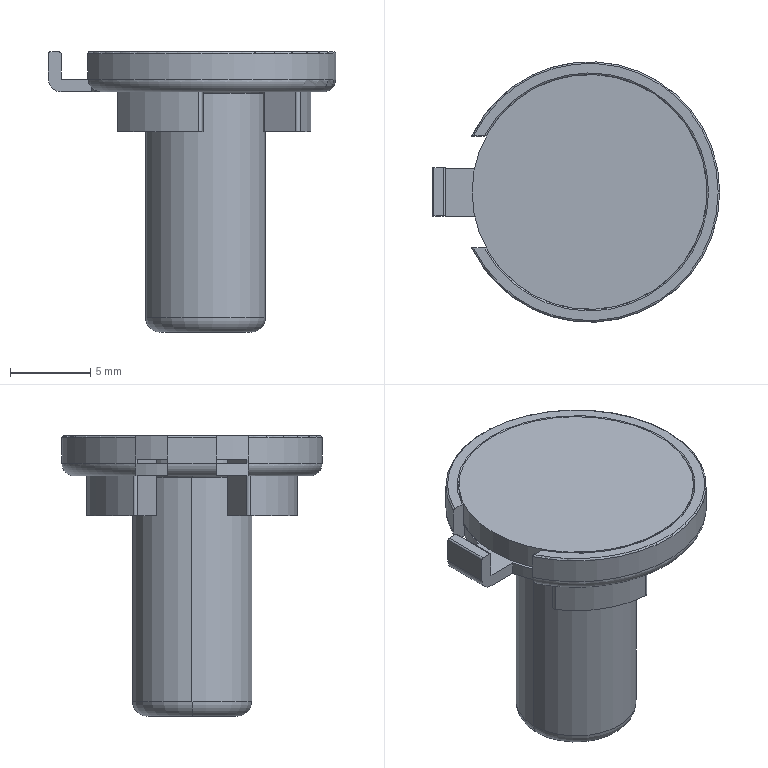NC program | NX | posted with a generic post | part box 17.958 x 16.273 x 17.5 mm
Lines 3567 to 4449 of 11029:
(ZLEVEL_PROFILE_COPY_COPY_2_COPY_1 , TOOL : D2)
N7126 T02 M6
N7128 G54
N7130 G17 G0 G90 X-1.219 Y-5.219 S8000 M3
N7132 G43 Z30. H2
N7134 Z-0.194
N7136 G94 G1 X-0.925 Y-5.036 F1000.
N7138 G3 X-0.831 Y-4.859 R0.2
N7140 G1 X-0.853 Y-4.228
N7142 G2 X-0.81 Y-3.866 R1.2
N7144 X-1.762 Y-3.535 R3.95
N7146 G3 X-1.961 Y-3.548 R0.2
N7148 G1 X-2.237 Y-3.731
N7150 G0 X-1.219 Y-5.219 Z-0.389
N7152 G1 X-0.925 Y-5.036
N7154 G3 X-0.831 Y-4.859 R0.2
N7156 G1 X-0.853 Y-4.228
N7158 G2 X-0.81 Y-3.866 R1.2
N7160 X-1.762 Y-3.535 R3.95
N7162 G3 X-1.961 Y-3.548 R0.2
N7164 G1 X-2.237 Y-3.731
N7166 G0 X-1.219 Y-5.219 Z-0.583
N7168 G1 X-0.925 Y-5.036
N7170 G3 X-0.831 Y-4.859 R0.2
N7172 G1 X-0.853 Y-4.228
N7174 G2 X-0.81 Y-3.866 R1.2
N7176 X-1.762 Y-3.535 R3.95
N7178 G3 X-1.961 Y-3.548 R0.2
N7180 G1 X-2.237 Y-3.731
N7182 G0 X-1.219 Y-5.219 Z-0.778
N7184 G1 X-0.925 Y-5.036
N7186 G3 X-0.831 Y-4.859 R0.2
N7188 G1 X-0.853 Y-4.228
N7190 G2 X-0.81 Y-3.866 R1.2
N7192 X-1.762 Y-3.535 R3.95
N7194 G3 X-1.961 Y-3.548 R0.2
N7196 G1 X-2.237 Y-3.731
N7198 G0 X-1.219 Y-5.219 Z-0.972
N7200 G1 X-0.925 Y-5.036
N7202 G3 X-0.831 Y-4.859 R0.2
N7204 G1 X-0.853 Y-4.228
N7206 G2 X-0.81 Y-3.866 R1.2
N7208 X-1.762 Y-3.535 R3.95
N7210 G3 X-1.961 Y-3.548 R0.2
N7212 G1 X-2.237 Y-3.731
N7214 G0 X-1.219 Y-5.219 Z-1.167
N7216 G1 X-0.925 Y-5.036
N7218 G3 X-0.831 Y-4.859 R0.2
N7220 G1 X-0.853 Y-4.228
N7222 G2 X-0.81 Y-3.866 R1.2
N7224 X-1.762 Y-3.535 R3.95
N7226 G3 X-1.961 Y-3.548 R0.2
N7228 G1 X-2.237 Y-3.731
N7230 G0 X-1.219 Y-5.219 Z-1.361
N7232 G1 X-0.925 Y-5.036
N7234 G3 X-0.831 Y-4.859 R0.2
N7236 G1 X-0.853 Y-4.228
N7238 G2 X-0.81 Y-3.866 R1.2
N7240 X-1.762 Y-3.535 R3.95
N7242 G3 X-1.961 Y-3.548 R0.2
N7244 G1 X-2.237 Y-3.731
N7246 G0 X-1.219 Y-5.219 Z-1.556
N7248 G1 X-0.925 Y-5.036
N7250 G3 X-0.831 Y-4.859 R0.2
N7252 G1 X-0.853 Y-4.228
N7254 G2 X-0.81 Y-3.866 R1.2
N7256 X-1.762 Y-3.535 R3.95
N7258 G3 X-1.961 Y-3.548 R0.2
N7260 G1 X-2.237 Y-3.731
N7262 G0 X-1.219 Y-5.219 Z-1.75
N7264 G1 X-0.925 Y-5.036
N7266 G3 X-0.831 Y-4.859 R0.2
N7268 G1 X-0.853 Y-4.228
N7270 G2 X-0.81 Y-3.866 R1.2
N7272 X-1.762 Y-3.535 R3.95
N7274 G3 X-1.961 Y-3.548 R0.2
N7276 G1 X-2.237 Y-3.731
N7278 G0 X-1.219 Y-5.219 Z-1.944
N7280 G1 X-0.925 Y-5.036
N7282 G3 X-0.831 Y-4.859 R0.2
N7284 G1 X-0.853 Y-4.228
N7286 G2 X-0.81 Y-3.866 R1.2
N7288 X-1.762 Y-3.535 R3.95
N7290 G3 X-1.961 Y-3.548 R0.2
N7292 G1 X-2.237 Y-3.731
N7294 G0 X-1.219 Y-5.219 Z-2.139
N7296 G1 X-0.925 Y-5.036
N7298 G3 X-0.831 Y-4.859 R0.2
N7300 G1 X-0.853 Y-4.228
N7302 G2 X-0.81 Y-3.866 R1.2
N7304 X-1.762 Y-3.535 R3.95
N7306 G3 X-1.961 Y-3.548 R0.2
N7308 G1 X-2.237 Y-3.731
N7310 G0 X-1.219 Y-5.219 Z-2.333
N7312 G1 X-0.925 Y-5.036
N7314 G3 X-0.831 Y-4.859 R0.2
N7316 G1 X-0.853 Y-4.228
N7318 G2 X-0.81 Y-3.866 R1.2
N7320 X-1.762 Y-3.535 R3.95
N7322 G3 X-1.961 Y-3.548 R0.2
N7324 G1 X-2.237 Y-3.731
N7326 G0 X-1.219 Y-5.219 Z-2.528
N7328 G1 X-0.925 Y-5.036
N7330 G3 X-0.831 Y-4.859 R0.2
N7332 G1 X-0.853 Y-4.228
N7334 G2 X-0.81 Y-3.866 R1.2
N7336 X-1.762 Y-3.535 R3.95
N7338 G3 X-1.961 Y-3.548 R0.2
N7340 G1 X-2.237 Y-3.731
N7342 G0 X-1.219 Y-5.219 Z-2.722
N7344 G1 X-0.925 Y-5.036
N7346 G3 X-0.831 Y-4.859 R0.2
N7348 G1 X-0.853 Y-4.228
N7350 G2 X-0.81 Y-3.866 R1.2
N7352 X-1.762 Y-3.535 R3.95
N7354 G3 X-1.961 Y-3.548 R0.2
N7356 G1 X-2.237 Y-3.73
N7358 G0 X-1.219 Y-5.219 Z-2.917
N7360 G1 X-0.925 Y-5.036
N7362 G3 X-0.831 Y-4.859 R0.2
N7364 G1 X-0.853 Y-4.228
N7366 G2 X-0.81 Y-3.866 R1.2
N7368 X-1.762 Y-3.535 R3.95
N7370 G3 X-1.961 Y-3.548 R0.2
N7372 G1 X-2.237 Y-3.73
N7374 G0 X-1.219 Y-5.219 Z-3.111
N7376 G1 X-0.925 Y-5.036
N7378 G3 X-0.831 Y-4.859 R0.2
N7380 G1 X-0.853 Y-4.228
N7382 G2 X-0.81 Y-3.866 R1.2
N7384 X-1.762 Y-3.535 R3.95
N7386 G3 X-1.961 Y-3.548 R0.2
N7388 G1 X-2.237 Y-3.73
N7390 G0 X-1.219 Y-5.219 Z-3.306
N7392 G1 X-0.925 Y-5.036
N7394 G3 X-0.831 Y-4.859 R0.2
N7396 G1 X-0.853 Y-4.228
N7398 G2 X-0.81 Y-3.866 R1.2
N7400 X-1.762 Y-3.535 R3.95
N7402 G3 X-1.961 Y-3.548 R0.2
N7404 G1 X-2.237 Y-3.73
N7406 G0 X-1.219 Y-5.219 Z-3.5
N7408 G1 X-0.925 Y-5.036
N7410 G3 X-0.831 Y-4.859 R0.2
N7412 G1 X-0.853 Y-4.228
N7414 G2 X-0.81 Y-3.866 R1.2
N7416 X-1.762 Y-3.535 R3.95
N7418 G3 X-1.961 Y-3.548 R0.2
N7420 G1 X-2.237 Y-3.73
N7422 G0 Z30.
N7424 X-2.112 Y-3.803
N7426 Z-0.194
N7428 G1 X-2.092 Y-3.472
N7430 G3 X-2.181 Y-3.293 R0.2
N7432 G2 X-2.943 Y-2.635 R3.95
N7434 X-3.235 Y-2.853 R1.2
N7436 G1 X-3.792 Y-3.149
N7438 G3 X-3.898 Y-3.319 R0.2
N7440 G1 X-3.911 Y-3.665
N7442 G0 X-2.112 Y-3.803 Z-0.389
N7444 G1 X-2.092 Y-3.472
N7446 G3 X-2.181 Y-3.293 R0.2
N7448 G2 X-2.943 Y-2.635 R3.95
N7450 X-3.235 Y-2.853 R1.2
N7452 G1 X-3.792 Y-3.149
N7454 G3 X-3.898 Y-3.319 R0.2
N7456 G1 X-3.911 Y-3.665
N7458 G0 X-2.112 Y-3.803 Z-0.583
N7460 G1 X-2.092 Y-3.472
N7462 G3 X-2.181 Y-3.293 R0.2
N7464 G2 X-2.943 Y-2.635 R3.95
N7466 X-3.235 Y-2.853 R1.2
N7468 G1 X-3.793 Y-3.149
N7470 G3 X-3.898 Y-3.319 R0.2
N7472 G1 X-3.911 Y-3.665
N7474 G0 X-2.112 Y-3.803 Z-0.778
N7476 G1 X-2.092 Y-3.472
N7478 G3 X-2.181 Y-3.293 R0.2
N7480 G2 X-2.943 Y-2.635 R3.95
N7482 X-3.235 Y-2.853 R1.2
N7484 G1 X-3.793 Y-3.149
N7486 G3 X-3.899 Y-3.319 R0.2
N7488 G1 X-3.911 Y-3.665
N7490 G0 X-2.112 Y-3.803 Z-0.972
N7492 G1 X-2.092 Y-3.472
N7494 G3 X-2.181 Y-3.293 R0.2
N7496 G2 X-2.943 Y-2.635 R3.95
N7498 X-3.235 Y-2.853 R1.2
N7500 G1 X-3.793 Y-3.149
N7502 G3 X-3.899 Y-3.319 R0.2
N7504 G1 X-3.911 Y-3.665
N7506 G0 X-2.112 Y-3.803 Z-1.167
N7508 G1 X-2.092 Y-3.472
N7510 G3 X-2.181 Y-3.293 R0.2
N7512 G2 X-2.943 Y-2.635 R3.95
N7514 X-3.235 Y-2.853 R1.2
N7516 G1 X-3.793 Y-3.149
N7518 G3 X-3.899 Y-3.319 R0.2
N7520 G1 X-3.911 Y-3.665
N7522 G0 X-2.112 Y-3.803 Z-1.361
N7524 G1 X-2.092 Y-3.472
N7526 G3 X-2.181 Y-3.293 R0.2
N7528 G2 X-2.943 Y-2.635 R3.95
N7530 X-3.235 Y-2.853 R1.2
N7532 G1 X-3.793 Y-3.149
N7534 G3 X-3.899 Y-3.319 R0.2
N7536 G1 X-3.911 Y-3.665
N7538 G0 X-2.112 Y-3.803 Z-1.556
N7540 G1 X-2.092 Y-3.472
N7542 G3 X-2.181 Y-3.293 R0.2
N7544 G2 X-2.943 Y-2.635 R3.95
N7546 X-3.235 Y-2.853 R1.2
N7548 G1 X-3.793 Y-3.149
N7550 G3 X-3.899 Y-3.319 R0.2
N7552 G1 X-3.911 Y-3.665
N7554 G0 X-2.112 Y-3.803 Z-1.75
N7556 G1 X-2.092 Y-3.472
N7558 G3 X-2.181 Y-3.293 R0.2
N7560 G2 X-2.943 Y-2.635 R3.95
N7562 X-3.235 Y-2.853 R1.2
N7564 G1 X-3.793 Y-3.149
N7566 G3 X-3.899 Y-3.319 R0.2
N7568 G1 X-3.911 Y-3.665
N7570 G0 X-2.112 Y-3.803 Z-1.944
N7572 G1 X-2.092 Y-3.472
N7574 G3 X-2.181 Y-3.293 R0.2
N7576 G2 X-2.943 Y-2.635 R3.95
N7578 X-3.235 Y-2.853 R1.2
N7580 G1 X-3.793 Y-3.149
N7582 G3 X-3.899 Y-3.319 R0.2
N7584 G1 X-3.911 Y-3.665
N7586 G0 X-2.112 Y-3.803 Z-2.139
N7588 G1 X-2.092 Y-3.472
N7590 G3 X-2.181 Y-3.293 R0.2
N7592 G2 X-2.943 Y-2.635 R3.95
N7594 X-3.235 Y-2.853 R1.2
N7596 G1 X-3.793 Y-3.149
N7598 G3 X-3.899 Y-3.319 R0.2
N7600 G1 X-3.911 Y-3.665
N7602 G0 X-2.112 Y-3.803 Z-2.333
N7604 G1 X-2.092 Y-3.472
N7606 G3 X-2.181 Y-3.293 R0.2
N7608 G2 X-2.943 Y-2.635 R3.95
N7610 X-3.235 Y-2.853 R1.2
N7612 G1 X-3.793 Y-3.149
N7614 G3 X-3.899 Y-3.319 R0.2
N7616 G1 X-3.911 Y-3.665
N7618 G0 X-2.112 Y-3.803 Z-2.528
N7620 G1 X-2.092 Y-3.472
N7622 G3 X-2.181 Y-3.293 R0.2
N7624 G2 X-2.943 Y-2.635 R3.95
N7626 X-3.235 Y-2.853 R1.2
N7628 G1 X-3.793 Y-3.149
N7630 G3 X-3.899 Y-3.319 R0.2
N7632 G1 X-3.911 Y-3.665
N7634 G0 X-2.112 Y-3.803 Z-2.722
N7636 G1 X-2.092 Y-3.472
N7638 G3 X-2.181 Y-3.293 R0.2
N7640 G2 X-2.943 Y-2.635 R3.95
N7642 X-3.235 Y-2.853 R1.2
N7644 G1 X-3.793 Y-3.149
N7646 G3 X-3.899 Y-3.319 R0.2
N7648 G1 X-3.911 Y-3.665
N7650 G0 X-2.112 Y-3.803 Z-2.917
N7652 G1 X-2.092 Y-3.472
N7654 G3 X-2.181 Y-3.293 R0.2
N7656 G2 X-2.943 Y-2.635 R3.95
N7658 X-3.235 Y-2.853 R1.2
N7660 G1 X-3.793 Y-3.149
N7662 G3 X-3.899 Y-3.319 R0.2
N7664 G1 X-3.911 Y-3.665
N7666 G0 X-2.112 Y-3.803 Z-3.111
N7668 G1 X-2.092 Y-3.472
N7670 G3 X-2.181 Y-3.293 R0.2
N7672 G2 X-2.943 Y-2.635 R3.95
N7674 X-3.235 Y-2.853 R1.2
N7676 G1 X-3.793 Y-3.149
N7678 G3 X-3.899 Y-3.319 R0.2
N7680 G1 X-3.911 Y-3.665
N7682 G0 X-2.112 Y-3.803 Z-3.306
N7684 G1 X-2.092 Y-3.472
N7686 G3 X-2.181 Y-3.293 R0.2
N7688 G2 X-2.943 Y-2.635 R3.95
N7690 X-3.235 Y-2.853 R1.2
N7692 G1 X-3.793 Y-3.149
N7694 G3 X-3.899 Y-3.319 R0.2
N7696 G1 X-3.911 Y-3.665
N7698 G0 X-2.112 Y-3.803 Z-3.5
N7700 G1 X-2.092 Y-3.472
N7702 G3 X-2.181 Y-3.293 R0.2
N7704 G2 X-2.943 Y-2.635 R3.95
N7706 X-3.235 Y-2.853 R1.2
N7708 G1 X-3.793 Y-3.149
N7710 G3 X-3.899 Y-3.319 R0.2
N7712 G1 X-3.911 Y-3.665
N7714 G0 Z30.
N7716 Y3.665
N7718 Z-0.194
N7720 G1 X-3.898 Y3.319
N7722 G3 X-3.792 Y3.149 R0.2
N7724 G1 X-3.235 Y2.853
N7726 G2 X-2.943 Y2.635 R1.2
N7728 X-2.181 Y3.293 R3.95
N7730 G3 X-2.092 Y3.472 R0.2
N7732 G1 X-2.112 Y3.803
N7734 G0 X-3.911 Y3.665 Z-0.389
N7736 G1 X-3.898 Y3.319
N7738 G3 X-3.792 Y3.149 R0.2
N7740 G1 X-3.235 Y2.853
N7742 G2 X-2.943 Y2.635 R1.2
N7744 X-2.181 Y3.293 R3.95
N7746 G3 X-2.092 Y3.472 R0.2
N7748 G1 X-2.112 Y3.803
N7750 G0 X-3.911 Y3.665 Z-0.583
N7752 G1 X-3.898 Y3.319
N7754 G3 X-3.793 Y3.149 R0.2
N7756 G1 X-3.235 Y2.853
N7758 G2 X-2.943 Y2.635 R1.2
N7760 X-2.181 Y3.293 R3.95
N7762 G3 X-2.092 Y3.472 R0.2
N7764 G1 X-2.112 Y3.803
N7766 G0 X-3.911 Y3.665 Z-0.778
N7768 G1 X-3.899 Y3.319
N7770 G3 X-3.793 Y3.149 R0.2
N7772 G1 X-3.235 Y2.853
N7774 G2 X-2.943 Y2.635 R1.2
N7776 X-2.181 Y3.293 R3.95
N7778 G3 X-2.092 Y3.472 R0.2
N7780 G1 X-2.112 Y3.803
N7782 G0 X-3.911 Y3.665 Z-0.972
N7784 G1 X-3.899 Y3.319
N7786 G3 X-3.793 Y3.149 R0.2
N7788 G1 X-3.235 Y2.853
N7790 G2 X-2.943 Y2.635 R1.2
N7792 X-2.181 Y3.293 R3.95
N7794 G3 X-2.092 Y3.472 R0.2
N7796 G1 X-2.112 Y3.803
N7798 G0 X-3.911 Y3.665 Z-1.167
N7800 G1 X-3.899 Y3.319
N7802 G3 X-3.793 Y3.149 R0.2
N7804 G1 X-3.235 Y2.853
N7806 G2 X-2.943 Y2.635 R1.2
N7808 X-2.181 Y3.293 R3.95
N7810 G3 X-2.092 Y3.472 R0.2
N7812 G1 X-2.112 Y3.803
N7814 G0 X-3.911 Y3.665 Z-1.361
N7816 G1 X-3.899 Y3.319
N7818 G3 X-3.793 Y3.149 R0.2
N7820 G1 X-3.235 Y2.853
N7822 G2 X-2.943 Y2.635 R1.2
N7824 X-2.181 Y3.293 R3.95
N7826 G3 X-2.092 Y3.472 R0.2
N7828 G1 X-2.112 Y3.803
N7830 G0 X-3.911 Y3.665 Z-1.556
N7832 G1 X-3.899 Y3.319
N7834 G3 X-3.793 Y3.149 R0.2
N7836 G1 X-3.235 Y2.853
N7838 G2 X-2.943 Y2.635 R1.2
N7840 X-2.181 Y3.293 R3.95
N7842 G3 X-2.092 Y3.472 R0.2
N7844 G1 X-2.112 Y3.803
N7846 G0 X-3.911 Y3.665 Z-1.75
N7848 G1 X-3.899 Y3.319
N7850 G3 X-3.793 Y3.149 R0.2
N7852 G1 X-3.235 Y2.853
N7854 G2 X-2.943 Y2.635 R1.2
N7856 X-2.181 Y3.293 R3.95
N7858 G3 X-2.092 Y3.472 R0.2
N7860 G1 X-2.112 Y3.803
N7862 G0 X-3.911 Y3.665 Z-1.944
N7864 G1 X-3.899 Y3.319
N7866 G3 X-3.793 Y3.149 R0.2
N7868 G1 X-3.235 Y2.853
N7870 G2 X-2.943 Y2.635 R1.2
N7872 X-2.181 Y3.293 R3.95
N7874 G3 X-2.092 Y3.472 R0.2
N7876 G1 X-2.112 Y3.803
N7878 G0 X-3.911 Y3.665 Z-2.139
N7880 G1 X-3.899 Y3.319
N7882 G3 X-3.793 Y3.149 R0.2
N7884 G1 X-3.235 Y2.853
N7886 G2 X-2.943 Y2.635 R1.2
N7888 X-2.181 Y3.293 R3.95
N7890 G3 X-2.092 Y3.472 R0.2
N7892 G1 X-2.112 Y3.803
N7894 G0 X-3.911 Y3.665 Z-2.333
N7896 G1 X-3.899 Y3.319
N7898 G3 X-3.793 Y3.149 R0.2
N7900 G1 X-3.235 Y2.853
N7902 G2 X-2.943 Y2.635 R1.2
N7904 X-2.181 Y3.293 R3.95
N7906 G3 X-2.092 Y3.472 R0.2
N7908 G1 X-2.112 Y3.803
N7910 G0 X-3.911 Y3.665 Z-2.528
N7912 G1 X-3.899 Y3.319
N7914 G3 X-3.793 Y3.149 R0.2
N7916 G1 X-3.235 Y2.853
N7918 G2 X-2.943 Y2.635 R1.2
N7920 X-2.181 Y3.293 R3.95
N7922 G3 X-2.092 Y3.472 R0.2
N7924 G1 X-2.112 Y3.803
N7926 G0 X-3.911 Y3.665 Z-2.722
N7928 G1 X-3.899 Y3.319
N7930 G3 X-3.793 Y3.149 R0.2
N7932 G1 X-3.235 Y2.853
N7934 G2 X-2.943 Y2.635 R1.2
N7936 X-2.181 Y3.293 R3.95
N7938 G3 X-2.092 Y3.472 R0.2
N7940 G1 X-2.112 Y3.803
N7942 G0 X-3.911 Y3.665 Z-2.917
N7944 G1 X-3.899 Y3.319
N7946 G3 X-3.793 Y3.149 R0.2
N7948 G1 X-3.235 Y2.853
N7950 G2 X-2.943 Y2.635 R1.2
N7952 X-2.181 Y3.293 R3.95
N7954 G3 X-2.092 Y3.472 R0.2
N7956 G1 X-2.112 Y3.803
N7958 G0 X-3.911 Y3.665 Z-3.111
N7960 G1 X-3.899 Y3.319
N7962 G3 X-3.793 Y3.149 R0.2
N7964 G1 X-3.235 Y2.853
N7966 G2 X-2.943 Y2.635 R1.2
N7968 X-2.181 Y3.293 R3.95
N7970 G3 X-2.092 Y3.472 R0.2
N7972 G1 X-2.112 Y3.803
N7974 G0 X-3.911 Y3.665 Z-3.306
N7976 G1 X-3.899 Y3.319
N7978 G3 X-3.793 Y3.149 R0.2
N7980 G1 X-3.235 Y2.853
N7982 G2 X-2.943 Y2.635 R1.2
N7984 X-2.181 Y3.293 R3.95
N7986 G3 X-2.092 Y3.472 R0.2
N7988 G1 X-2.112 Y3.803
N7990 G0 X-3.911 Y3.665 Z-3.5
N7992 G1 X-3.899 Y3.319
N7994 G3 X-3.793 Y3.149 R0.2
N7996 G1 X-3.235 Y2.853
N7998 G2 X-2.943 Y2.635 R1.2
N8000 X-2.181 Y3.293 R3.95
N8002 G3 X-2.092 Y3.472 R0.2
N8004 G1 X-2.112 Y3.803
N8006 G0 Z30.
N8008 X-2.237 Y3.731
N8010 Z-0.194
N8012 G1 X-1.961 Y3.548
N8014 G3 X-1.762 Y3.535 R0.2
N8016 G2 X-0.81 Y3.866 R3.95
N8018 X-0.853 Y4.228 R1.2
N8020 G1 X-0.831 Y4.859
N8022 G3 X-0.925 Y5.036 R0.2
N8024 G1 X-1.219 Y5.219
N8026 G0 X-2.237 Y3.731 Z-0.389
N8028 G1 X-1.961 Y3.548
N8030 G3 X-1.762 Y3.535 R0.2
N8032 G2 X-0.81 Y3.866 R3.95
N8034 X-0.853 Y4.228 R1.2
N8036 G1 X-0.831 Y4.859
N8038 G3 X-0.925 Y5.036 R0.2
N8040 G1 X-1.219 Y5.219
N8042 G0 X-2.237 Y3.731 Z-0.583
N8044 G1 X-1.961 Y3.548
N8046 G3 X-1.762 Y3.535 R0.2
N8048 G2 X-0.81 Y3.866 R3.95
N8050 X-0.853 Y4.228 R1.2
N8052 G1 X-0.831 Y4.859
N8054 G3 X-0.925 Y5.036 R0.2
N8056 G1 X-1.219 Y5.219
N8058 G0 X-2.237 Y3.731 Z-0.778
N8060 G1 X-1.961 Y3.548
N8062 G3 X-1.762 Y3.535 R0.2
N8064 G2 X-0.81 Y3.866 R3.95
N8066 X-0.853 Y4.228 R1.2
N8068 G1 X-0.831 Y4.859
N8070 G3 X-0.925 Y5.036 R0.2
N8072 G1 X-1.219 Y5.219
N8074 G0 X-2.237 Y3.731 Z-0.972
N8076 G1 X-1.961 Y3.548
N8078 G3 X-1.762 Y3.535 R0.2
N8080 G2 X-0.81 Y3.866 R3.95
N8082 X-0.853 Y4.228 R1.2
N8084 G1 X-0.831 Y4.859
N8086 G3 X-0.925 Y5.036 R0.2
N8088 G1 X-1.219 Y5.219
N8090 G0 X-2.237 Y3.731 Z-1.167
N8092 G1 X-1.961 Y3.548
N8094 G3 X-1.762 Y3.535 R0.2
N8096 G2 X-0.81 Y3.866 R3.95
N8098 X-0.853 Y4.228 R1.2
N8100 G1 X-0.831 Y4.859
N8102 G3 X-0.925 Y5.036 R0.2
N8104 G1 X-1.219 Y5.219
N8106 G0 X-2.237 Y3.731 Z-1.361
N8108 G1 X-1.961 Y3.548
N8110 G3 X-1.762 Y3.535 R0.2
N8112 G2 X-0.81 Y3.866 R3.95
N8114 X-0.853 Y4.228 R1.2
N8116 G1 X-0.831 Y4.859
N8118 G3 X-0.925 Y5.036 R0.2
N8120 G1 X-1.219 Y5.219
N8122 G0 X-2.237 Y3.731 Z-1.556
N8124 G1 X-1.961 Y3.548
N8126 G3 X-1.762 Y3.535 R0.2
N8128 G2 X-0.811 Y3.866 R3.95
N8130 X-0.853 Y4.228 R1.2
N8132 G1 X-0.831 Y4.859
N8134 G3 X-0.925 Y5.036 R0.2
N8136 G1 X-1.219 Y5.219
N8138 G0 X-2.237 Y3.731 Z-1.75
N8140 G1 X-1.961 Y3.548
N8142 G3 X-1.762 Y3.535 R0.2
N8144 G2 X-0.811 Y3.866 R3.95
N8146 X-0.853 Y4.228 R1.2
N8148 G1 X-0.831 Y4.859
N8150 G3 X-0.925 Y5.036 R0.2
N8152 G1 X-1.219 Y5.219
N8154 G0 X-2.237 Y3.731 Z-1.944
N8156 G1 X-1.961 Y3.548
N8158 G3 X-1.762 Y3.535 R0.2
N8160 G2 X-0.811 Y3.866 R3.95
N8162 X-0.853 Y4.228 R1.2
N8164 G1 X-0.831 Y4.859
N8166 G3 X-0.925 Y5.036 R0.2
N8168 G1 X-1.219 Y5.219
N8170 G0 X-2.237 Y3.731 Z-2.139
N8172 G1 X-1.961 Y3.548
N8174 G3 X-1.762 Y3.535 R0.2
N8176 G2 X-0.811 Y3.866 R3.95
N8178 X-0.853 Y4.228 R1.2
N8180 G1 X-0.831 Y4.859
N8182 G3 X-0.925 Y5.036 R0.2
N8184 G1 X-1.219 Y5.219
N8186 G0 X-2.237 Y3.731 Z-2.333
N8188 G1 X-1.961 Y3.548
N8190 G3 X-1.762 Y3.535 R0.2
N8192 G2 X-0.811 Y3.866 R3.95
N8194 X-0.853 Y4.228 R1.2
N8196 G1 X-0.831 Y4.859
N8198 G3 X-0.925 Y5.036 R0.2
N8200 G1 X-1.219 Y5.219
N8202 G0 X-2.237 Y3.731 Z-2.528
N8204 G1 X-1.961 Y3.548
N8206 G3 X-1.762 Y3.535 R0.2
N8208 G2 X-0.811 Y3.866 R3.95
N8210 X-0.853 Y4.228 R1.2
N8212 G1 X-0.831 Y4.859
N8214 G3 X-0.925 Y5.036 R0.2
N8216 G1 X-1.219 Y5.219
N8218 G0 X-2.237 Y3.731 Z-2.722
N8220 G1 X-1.961 Y3.548
N8222 G3 X-1.762 Y3.535 R0.2
N8224 G2 X-0.811 Y3.866 R3.95
N8226 X-0.853 Y4.228 R1.2
N8228 G1 X-0.831 Y4.859
N8230 G3 X-0.925 Y5.036 R0.2
N8232 G1 X-1.219 Y5.219
N8234 G0 X-2.237 Y3.731 Z-2.917
N8236 G1 X-1.961 Y3.548
N8238 G3 X-1.762 Y3.535 R0.2
N8240 G2 X-0.811 Y3.866 R3.95
N8242 X-0.853 Y4.228 R1.2
N8244 G1 X-0.831 Y4.859
N8246 G3 X-0.925 Y5.036 R0.2
N8248 G1 X-1.219 Y5.219
N8250 G0 X-2.237 Y3.731 Z-3.111
N8252 G1 X-1.961 Y3.548
N8254 G3 X-1.762 Y3.535 R0.2
N8256 G2 X-0.811 Y3.866 R3.95
N8258 X-0.853 Y4.228 R1.2
N8260 G1 X-0.831 Y4.859
N8262 G3 X-0.925 Y5.036 R0.2
N8264 G1 X-1.219 Y5.219
N8266 G0 X-2.237 Y3.731 Z-3.306
N8268 G1 X-1.961 Y3.548
N8270 G3 X-1.762 Y3.535 R0.2
N8272 G2 X-0.811 Y3.866 R3.95
N8274 X-0.853 Y4.228 R1.2
N8276 G1 X-0.831 Y4.859
N8278 G3 X-0.925 Y5.036 R0.2
N8280 G1 X-1.219 Y5.219
N8282 G0 X-2.237 Y3.731 Z-3.5
N8284 G1 X-1.961 Y3.548
N8286 G3 X-1.762 Y3.535 R0.2
N8288 G2 X-0.811 Y3.866 R3.95
N8290 X-0.853 Y4.228 R1.2
N8292 G1 X-0.831 Y4.859
N8294 G3 X-0.925 Y5.036 R0.2
N8296 G1 X-1.219 Y5.219
N8298 G0 Z30.
N8300 X5.129 Y1.554
N8302 Z-0.194
N8304 G1 X4.823 Y1.717
N8306 G3 X4.623 Y1.71 R0.2
N8308 G1 X4.088 Y1.375
N8310 G2 X3.753 Y1.231 R1.2
N8312 X3.943 Y0.242 R3.95
N8314 G3 X4.053 Y0.075 R0.2
N8316 G1 X4.349 Y-0.072
N8318 G0 X5.129 Y1.554 Z-0.389
N8320 G1 X4.823 Y1.717
N8322 G3 X4.623 Y1.71 R0.2
N8324 G1 X4.088 Y1.375
N8326 G2 X3.753 Y1.231 R1.2
N8328 X3.943 Y0.242 R3.95
N8330 G3 X4.053 Y0.075 R0.2
N8332 G1 X4.349 Y-0.072
N8334 G0 X5.129 Y1.554 Z-0.583
N8336 G1 X4.823 Y1.717
N8338 G3 X4.623 Y1.71 R0.2
N8340 G1 X4.088 Y1.375
N8342 G2 X3.753 Y1.231 R1.2
N8344 X3.943 Y0.242 R3.95
N8346 G3 X4.053 Y0.075 R0.2
N8348 G1 X4.349 Y-0.072
N8350 G0 X5.129 Y1.554 Z-0.778
N8352 G1 X4.823 Y1.717
N8354 G3 X4.623 Y1.71 R0.2
N8356 G1 X4.088 Y1.375
N8358 G2 X3.753 Y1.231 R1.2
N8360 X3.943 Y0.242 R3.95
N8362 G3 X4.053 Y0.075 R0.2
N8364 G1 X4.349 Y-0.072
N8366 G0 X5.129 Y1.554 Z-0.972
N8368 G1 X4.823 Y1.717
N8370 G3 X4.623 Y1.71 R0.2
N8372 G1 X4.088 Y1.375
N8374 G2 X3.753 Y1.231 R1.2
N8376 X3.943 Y0.242 R3.95
N8378 G3 X4.053 Y0.075 R0.2
N8380 G1 X4.349 Y-0.072
N8382 G0 X5.129 Y1.554 Z-1.167
N8384 G1 X4.823 Y1.717
N8386 G3 X4.623 Y1.71 R0.2
N8388 G1 X4.088 Y1.375
N8390 G2 X3.753 Y1.231 R1.2
N8392 X3.943 Y0.242 R3.95
N8394 G3 X4.053 Y0.075 R0.2
N8396 G1 X4.349 Y-0.072
N8398 G0 X5.129 Y1.554 Z-1.361
N8400 G1 X4.823 Y1.717
N8402 G3 X4.623 Y1.71 R0.2
N8404 G1 X4.088 Y1.375
N8406 G2 X3.753 Y1.231 R1.2
N8408 X3.943 Y0.242 R3.95
N8410 G3 X4.053 Y0.075 R0.2
N8412 G1 X4.349 Y-0.072
N8414 G0 X5.129 Y1.554 Z-1.556
N8416 G1 X4.823 Y1.717
N8418 G3 X4.623 Y1.71 R0.2
N8420 G1 X4.088 Y1.375
N8422 G2 X3.753 Y1.231 R1.2
N8424 X3.943 Y0.242 R3.95
N8426 G3 X4.053 Y0.075 R0.2
N8428 G1 X4.349 Y-0.072
N8430 G0 X5.129 Y1.554 Z-1.75
N8432 G1 X4.823 Y1.717
N8434 G3 X4.623 Y1.71 R0.2
N8436 G1 X4.088 Y1.375
N8438 G2 X3.753 Y1.231 R1.2
N8440 X3.943 Y0.242 R3.95
N8442 G3 X4.053 Y0.075 R0.2
N8444 G1 X4.349 Y-0.072
N8446 G0 X5.129 Y1.554 Z-1.944
N8448 G1 X4.823 Y1.717
N8450 G3 X4.623 Y1.71 R0.2
N8452 G1 X4.088 Y1.375
N8454 G2 X3.753 Y1.231 R1.2
N8456 X3.943 Y0.242 R3.95
N8458 G3 X4.053 Y0.075 R0.2
N8460 G1 X4.349 Y-0.072
N8462 G0 X5.129 Y1.554 Z-2.139
N8464 G1 X4.823 Y1.717
N8466 G3 X4.623 Y1.71 R0.2
N8468 G1 X4.088 Y1.375
N8470 G2 X3.753 Y1.231 R1.2
N8472 X3.943 Y0.242 R3.95
N8474 G3 X4.053 Y0.075 R0.2
N8476 G1 X4.349 Y-0.072
N8478 G0 X5.129 Y1.554 Z-2.333
N8480 G1 X4.823 Y1.717
N8482 G3 X4.623 Y1.71 R0.2
N8484 G1 X4.088 Y1.375
N8486 G2 X3.753 Y1.231 R1.2
N8488 X3.943 Y0.242 R3.95
N8490 G3 X4.053 Y0.075 R0.2
N8492 G1 X4.349 Y-0.072
N8494 G0 X5.129 Y1.554 Z-2.528
N8496 G1 X4.823 Y1.717
N8498 G3 X4.623 Y1.71 R0.2
N8500 G1 X4.088 Y1.375
N8502 G2 X3.753 Y1.231 R1.2
N8504 X3.943 Y0.242 R3.95
N8506 G3 X4.053 Y0.075 R0.2
N8508 G1 X4.349 Y-0.072
N8510 G0 X5.129 Y1.554 Z-2.722
N8512 G1 X4.823 Y1.717
N8514 G3 X4.623 Y1.71 R0.2
N8516 G1 X4.088 Y1.375
N8518 G2 X3.753 Y1.231 R1.2
N8520 X3.943 Y0.242 R3.95
N8522 G3 X4.053 Y0.075 R0.2
N8524 G1 X4.349 Y-0.072
N8526 G0 X5.129 Y1.554 Z-2.917
N8528 G1 X4.823 Y1.717
N8530 G3 X4.623 Y1.71 R0.2
N8532 G1 X4.088 Y1.375
N8534 G2 X3.753 Y1.231 R1.2
N8536 X3.943 Y0.242 R3.95
N8538 G3 X4.053 Y0.075 R0.2
N8540 G1 X4.349 Y-0.072
N8542 G0 X5.129 Y1.554 Z-3.111
N8544 G1 X4.823 Y1.717
N8546 G3 X4.623 Y1.71 R0.2
N8548 G1 X4.088 Y1.375
N8550 G2 X3.753 Y1.231 R1.2
N8552 X3.943 Y0.242 R3.95
N8554 G3 X4.053 Y0.075 R0.2
N8556 G1 X4.349 Y-0.072
N8558 G0 X5.129 Y1.554 Z-3.306
N8560 G1 X4.823 Y1.717
N8562 G3 X4.623 Y1.71 R0.2
N8564 G1 X4.088 Y1.375
N8566 G2 X3.753 Y1.231 R1.2
N8568 X3.943 Y0.242 R3.95
N8570 G3 X4.053 Y0.075 R0.2
N8572 G1 X4.349 Y-0.072
N8574 G0 X5.129 Y1.554 Z-3.5
N8576 G1 X4.823 Y1.717
N8578 G3 X4.623 Y1.71 R0.2
N8580 G1 X4.088 Y1.375
N8582 G2 X3.753 Y1.231 R1.2
N8584 X3.943 Y0.242 R3.95
N8586 G3 X4.053 Y0.075 R0.2
N8588 G1 X4.349 Y-0.072
N8590 G0 Z30.
N8592 Y0.072
N8594 Z-0.194
N8596 G1 X4.053 Y-0.075
N8598 G3 X3.943 Y-0.242 R0.2
N8600 G2 X3.753 Y-1.231 R3.95
N8602 X4.088 Y-1.375 R1.2
N8604 G1 X4.623 Y-1.71
N8606 G3 X4.823 Y-1.717 R0.2
N8608 G1 X5.129 Y-1.554
N8610 G0 X4.349 Y0.072 Z-0.389
N8612 G1 X4.053 Y-0.075
N8614 G3 X3.943 Y-0.242 R0.2
N8616 G2 X3.753 Y-1.231 R3.95
N8618 X4.088 Y-1.375 R1.2
N8620 G1 X4.623 Y-1.71
N8622 G3 X4.823 Y-1.717 R0.2
N8624 G1 X5.129 Y-1.554
N8626 G0 X4.349 Y0.072 Z-0.583
N8628 G1 X4.053 Y-0.075
N8630 G3 X3.943 Y-0.242 R0.2
N8632 G2 X3.753 Y-1.231 R3.95
N8634 X4.088 Y-1.375 R1.2
N8636 G1 X4.623 Y-1.71
N8638 G3 X4.823 Y-1.717 R0.2
N8640 G1 X5.129 Y-1.554
N8642 G0 X4.349 Y0.072 Z-0.778
N8644 G1 X4.053 Y-0.075
N8646 G3 X3.943 Y-0.242 R0.2
N8648 G2 X3.753 Y-1.231 R3.95
N8650 X4.088 Y-1.375 R1.2
N8652 G1 X4.623 Y-1.71
N8654 G3 X4.823 Y-1.717 R0.2
N8656 G1 X5.129 Y-1.554
N8658 G0 X4.349 Y0.072 Z-0.972
N8660 G1 X4.053 Y-0.075
N8662 G3 X3.943 Y-0.242 R0.2
N8664 G2 X3.753 Y-1.231 R3.95
N8666 X4.088 Y-1.375 R1.2
N8668 G1 X4.623 Y-1.71
N8670 G3 X4.823 Y-1.717 R0.2
N8672 G1 X5.129 Y-1.554
N8674 G0 X4.349 Y0.072 Z-1.167
N8676 G1 X4.053 Y-0.075
N8678 G3 X3.943 Y-0.242 R0.2
N8680 G2 X3.753 Y-1.231 R3.95
N8682 X4.088 Y-1.375 R1.2
N8684 G1 X4.623 Y-1.71
N8686 G3 X4.823 Y-1.717 R0.2
N8688 G1 X5.129 Y-1.554
N8690 G0 X4.349 Y0.072 Z-1.361
N8692 G1 X4.053 Y-0.075
N8694 G3 X3.943 Y-0.242 R0.2
N8696 G2 X3.753 Y-1.231 R3.95
N8698 X4.088 Y-1.375 R1.2
N8700 G1 X4.623 Y-1.71
N8702 G3 X4.823 Y-1.717 R0.2
N8704 G1 X5.129 Y-1.554
N8706 G0 X4.349 Y0.072 Z-1.556
N8708 G1 X4.053 Y-0.075
N8710 G3 X3.943 Y-0.242 R0.2
N8712 G2 X3.753 Y-1.231 R3.95
N8714 X4.088 Y-1.375 R1.2
N8716 G1 X4.623 Y-1.71
N8718 G3 X4.823 Y-1.717 R0.2
N8720 G1 X5.129 Y-1.554
N8722 G0 X4.349 Y0.072 Z-1.75
N8724 G1 X4.053 Y-0.075
N8726 G3 X3.943 Y-0.242 R0.2
N8728 G2 X3.753 Y-1.231 R3.95
N8730 X4.088 Y-1.375 R1.2
N8732 G1 X4.623 Y-1.71
N8734 G3 X4.823 Y-1.717 R0.2
N8736 G1 X5.129 Y-1.554
N8738 G0 X4.349 Y0.072 Z-1.944
N8740 G1 X4.053 Y-0.075
N8742 G3 X3.943 Y-0.242 R0.2
N8744 G2 X3.753 Y-1.231 R3.95
N8746 X4.088 Y-1.375 R1.2
N8748 G1 X4.623 Y-1.71
N8750 G3 X4.823 Y-1.717 R0.2
N8752 G1 X5.129 Y-1.554
N8754 G0 X4.349 Y0.072 Z-2.139
N8756 G1 X4.053 Y-0.075
N8758 G3 X3.943 Y-0.242 R0.2
N8760 G2 X3.753 Y-1.231 R3.95
N8762 X4.088 Y-1.375 R1.2
N8764 G1 X4.623 Y-1.71
N8766 G3 X4.823 Y-1.717 R0.2
N8768 G1 X5.129 Y-1.554
N8770 G0 X4.349 Y0.072 Z-2.333
N8772 G1 X4.053 Y-0.075
N8774 G3 X3.943 Y-0.242 R0.2
N8776 G2 X3.753 Y-1.231 R3.95
N8778 X4.088 Y-1.375 R1.2
N8780 G1 X4.623 Y-1.71
N8782 G3 X4.823 Y-1.717 R0.2
N8784 G1 X5.129 Y-1.554
N8786 G0 X4.349 Y0.072 Z-2.528
N8788 G1 X4.053 Y-0.075
N8790 G3 X3.943 Y-0.242 R0.2
N8792 G2 X3.753 Y-1.231 R3.95
N8794 X4.088 Y-1.375 R1.2
N8796 G1 X4.623 Y-1.71
N8798 G3 X4.823 Y-1.717 R0.2
N8800 G1 X5.129 Y-1.554
N8802 G0 X4.349 Y0.072 Z-2.722
N8804 G1 X4.053 Y-0.075
N8806 G3 X3.943 Y-0.242 R0.2
N8808 G2 X3.753 Y-1.231 R3.95
N8810 X4.088 Y-1.375 R1.2
N8812 G1 X4.623 Y-1.71
N8814 G3 X4.823 Y-1.717 R0.2
N8816 G1 X5.129 Y-1.554
N8818 G0 X4.349 Y0.072 Z-2.917
N8820 G1 X4.053 Y-0.075
N8822 G3 X3.943 Y-0.242 R0.2
N8824 G2 X3.753 Y-1.231 R3.95
N8826 X4.088 Y-1.375 R1.2
N8828 G1 X4.623 Y-1.71
N8830 G3 X4.823 Y-1.717 R0.2
N8832 G1 X5.129 Y-1.554
N8834 G0 X4.349 Y0.072 Z-3.111
N8836 G1 X4.053 Y-0.075
N8838 G3 X3.943 Y-0.242 R0.2
N8840 G2 X3.753 Y-1.231 R3.95
N8842 X4.088 Y-1.375 R1.2
N8844 G1 X4.623 Y-1.71
N8846 G3 X4.823 Y-1.717 R0.2
N8848 G1 X5.129 Y-1.554
N8850 G0 X4.349 Y0.072 Z-3.306
N8852 G1 X4.053 Y-0.075
N8854 G3 X3.943 Y-0.242 R0.2
N8856 G2 X3.753 Y-1.231 R3.95
N8858 X4.088 Y-1.375 R1.2
N8860 G1 X4.623 Y-1.71
N8862 G3 X4.823 Y-1.717 R0.2
N8864 G1 X5.129 Y-1.554
N8866 G0 X4.349 Y0.072 Z-3.5
N8868 G1 X4.053 Y-0.075
N8870 G3 X3.943 Y-0.242 R0.2
N8872 G2 X3.753 Y-1.231 R3.95
N8874 X4.088 Y-1.375 R1.2
N8876 G1 X4.623 Y-1.71
N8878 G3 X4.823 Y-1.717 R0.2
N8880 G1 X5.129 Y-1.554
N8882 G0 Z30.
N8884 M5